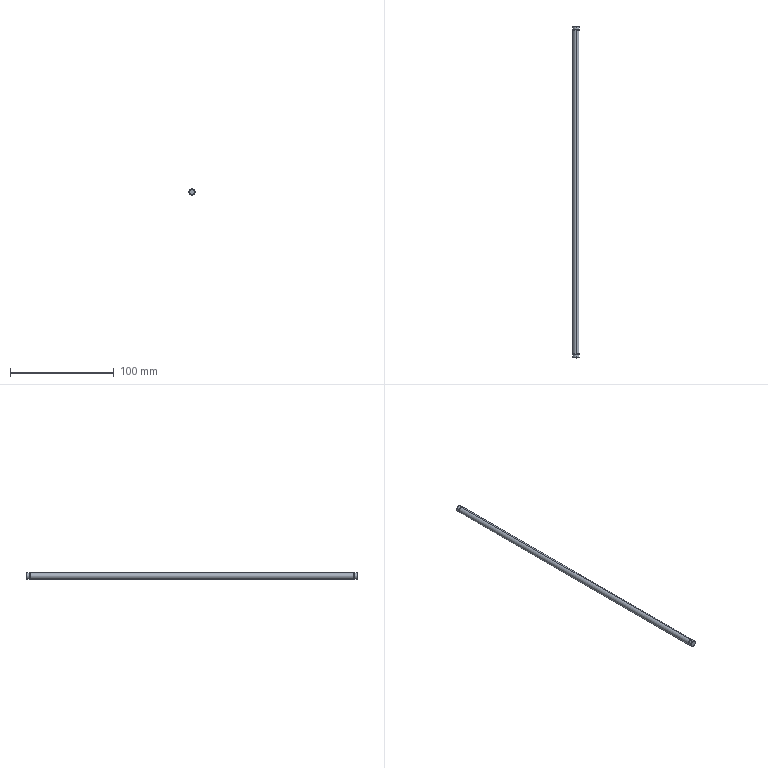Part | STEP file | 6mm pin shaft 001 | 1 solid | 20 faces | box 6 x 320 x 6 mm | volume 9038 mm3 | cylinder 10 | plane 6 | cone 4 | commonest cylinder face diameters 6 x6 5.6 x4
STEP:
#1=CARTESIAN_POINT('',(0.,0.,0.));
#2=DIRECTION('',(0.,0.,1.));
#3=DIRECTION('',(1.,0.,0.));
#4=AXIS2_PLACEMENT_3D('',#1,#2,#3);
#5=CARTESIAN_POINT('',(0.,-160.,-2.5));
#6=VERTEX_POINT('',#5);
#7=CARTESIAN_POINT('',(0.,-160.,2.5));
#8=VERTEX_POINT('',#7);
#9=CARTESIAN_POINT('',(0.,-160.,0.));
#10=DIRECTION('',(0.,-1.,0.));
#11=DIRECTION('',(0.,0.,1.));
#12=AXIS2_PLACEMENT_3D('',#9,#10,#11);
#13=CIRCLE('',#12,2.5);
#14=CARTESIAN_POINT('',(0.,-159.5,0.));
#15=DIRECTION('',(0.,1.,0.));
#16=DIRECTION('',(0.,0.,1.));
#17=AXIS2_PLACEMENT_3D('',#14,#15,#16);
#18=CONICAL_SURFACE('',#17,3.,0.7854);
#19=CARTESIAN_POINT('',(6.283,-0.5));
#20=DIRECTION('',(-1.,0.));
#21=VECTOR('',#20,1.);
#22=LINE('',#19,#21);
#23=(GEOMETRIC_REPRESENTATION_CONTEXT(2)PARAMETRIC_REPRESENTATION_CONTEXT()REPRESENTATION_CONTEXT('',''));
#24=DEFINITIONAL_REPRESENTATION('',(#22),#23);
#25=PCURVE('',#18,#24);
#26=CARTESIAN_POINT('',(0.,-160.,0.));
#27=DIRECTION('',(0.,1.,0.));
#28=DIRECTION('',(0.,0.,1.));
#29=AXIS2_PLACEMENT_3D('',#26,#27,#28);
#30=PLANE('',#29);
#31=CARTESIAN_POINT('',(2.5,0.));
#32=CARTESIAN_POINT('',(2.5,-4.33));
#33=CARTESIAN_POINT('',(-1.25,-2.165));
#34=CARTESIAN_POINT('',(-5.,0.));
#35=CARTESIAN_POINT('',(-1.25,2.165));
#36=CARTESIAN_POINT('',(2.5,4.33));
#37=CARTESIAN_POINT('',(2.5,0.));
#38=(BOUNDED_CURVE()B_SPLINE_CURVE(2,(#31,#32,#33,#34,#35,#36,#37),.UNSPECIFIED.,.T.,.F.)B_SPLINE_CURVE_WITH_KNOTS((1,2,2,2,2,1),(-2.094,0.,2.094,4.189,6.283,8.378),.UNSPECIFIED.)CURVE()GEOMETRIC_REPRESENTATION_ITEM()RATIONAL_B_SPLINE_CURVE((1.,0.5,1.,0.5,1.,0.5,1.))REPRESENTATION_ITEM(''));
#39=(GEOMETRIC_REPRESENTATION_CONTEXT(2)PARAMETRIC_REPRESENTATION_CONTEXT()REPRESENTATION_CONTEXT('',''));
#40=DEFINITIONAL_REPRESENTATION('',(#38),#39);
#41=PCURVE('',#30,#40);
#42=SURFACE_CURVE('',#13,(#25,#41),.PCURVE_S1.);
#43=EDGE_CURVE('',#6,#8,#42,.T.);
#44=ORIENTED_EDGE('',*,*,#43,.F.);
#45=CARTESIAN_POINT('',(0.,-159.5,-3.));
#46=VERTEX_POINT('',#45);
#47=CARTESIAN_POINT('',(0.,-159.5,-3.));
#48=DIRECTION('',(0.,0.7071,-0.7071));
#49=VECTOR('',#48,1.);
#50=LINE('',#47,#49);
#51=CARTESIAN_POINT('',(3.142,0.));
#52=DIRECTION('',(0.,1.));
#53=VECTOR('',#52,1.);
#54=LINE('',#51,#53);
#55=(GEOMETRIC_REPRESENTATION_CONTEXT(2)PARAMETRIC_REPRESENTATION_CONTEXT()REPRESENTATION_CONTEXT('',''));
#56=DEFINITIONAL_REPRESENTATION('',(#54),#55);
#57=PCURVE('',#18,#56);
#58=CARTESIAN_POINT('',(0.,-159.5,0.));
#59=DIRECTION('',(0.,1.,0.));
#60=DIRECTION('',(0.,0.,1.));
#61=AXIS2_PLACEMENT_3D('',#58,#59,#60);
#62=CONICAL_SURFACE('',#61,3.,0.7854);
#63=CARTESIAN_POINT('',(3.142,0.));
#64=DIRECTION('',(0.,1.));
#65=VECTOR('',#64,1.);
#66=LINE('',#63,#65);
#67=(GEOMETRIC_REPRESENTATION_CONTEXT(2)PARAMETRIC_REPRESENTATION_CONTEXT()REPRESENTATION_CONTEXT('',''));
#68=DEFINITIONAL_REPRESENTATION('',(#66),#67);
#69=PCURVE('',#62,#68);
#70=SURFACE_CURVE('',#50,(#57,#69),.PCURVE_S1.);
#71=EDGE_CURVE('',#6,#46,#70,.T.);
#72=ORIENTED_EDGE('',*,*,#71,.T.);
#73=CARTESIAN_POINT('',(0.,-159.5,3.));
#74=VERTEX_POINT('',#73);
#75=CARTESIAN_POINT('',(0.,-159.5,0.));
#76=DIRECTION('',(0.,1.,0.));
#77=DIRECTION('',(0.,0.,1.));
#78=AXIS2_PLACEMENT_3D('',#75,#76,#77);
#79=CIRCLE('',#78,3.);
#80=CARTESIAN_POINT('',(0.,0.));
#81=DIRECTION('',(1.,0.));
#82=VECTOR('',#81,1.);
#83=LINE('',#80,#82);
#84=(GEOMETRIC_REPRESENTATION_CONTEXT(2)PARAMETRIC_REPRESENTATION_CONTEXT()REPRESENTATION_CONTEXT('',''));
#85=DEFINITIONAL_REPRESENTATION('',(#83),#84);
#86=PCURVE('',#18,#85);
#87=CARTESIAN_POINT('',(0.,160.,0.));
#88=DIRECTION('',(0.,-1.,0.));
#89=DIRECTION('',(0.,0.,-1.));
#90=AXIS2_PLACEMENT_3D('',#87,#88,#89);
#91=CYLINDRICAL_SURFACE('',#90,3.);
#92=CARTESIAN_POINT('',(3.142,319.5));
#93=DIRECTION('',(-1.,0.));
#94=VECTOR('',#93,1.);
#95=LINE('',#92,#94);
#96=(GEOMETRIC_REPRESENTATION_CONTEXT(2)PARAMETRIC_REPRESENTATION_CONTEXT()REPRESENTATION_CONTEXT('',''));
#97=DEFINITIONAL_REPRESENTATION('',(#95),#96);
#98=PCURVE('',#91,#97);
#99=SURFACE_CURVE('',#79,(#86,#98),.PCURVE_S1.);
#100=EDGE_CURVE('',#74,#46,#99,.T.);
#101=ORIENTED_EDGE('',*,*,#100,.F.);
#102=CARTESIAN_POINT('',(0.,-159.5,3.));
#103=DIRECTION('',(0.,0.7071,0.7071));
#104=VECTOR('',#103,1.);
#105=LINE('',#102,#104);
#106=CARTESIAN_POINT('',(0.,0.));
#107=DIRECTION('',(0.,1.));
#108=VECTOR('',#107,1.);
#109=LINE('',#106,#108);
#110=(GEOMETRIC_REPRESENTATION_CONTEXT(2)PARAMETRIC_REPRESENTATION_CONTEXT()REPRESENTATION_CONTEXT('',''));
#111=DEFINITIONAL_REPRESENTATION('',(#109),#110);
#112=PCURVE('',#18,#111);
#113=CARTESIAN_POINT('',(6.283,0.));
#114=DIRECTION('',(0.,1.));
#115=VECTOR('',#114,1.);
#116=LINE('',#113,#115);
#117=(GEOMETRIC_REPRESENTATION_CONTEXT(2)PARAMETRIC_REPRESENTATION_CONTEXT()REPRESENTATION_CONTEXT('',''));
#118=DEFINITIONAL_REPRESENTATION('',(#116),#117);
#119=PCURVE('',#62,#118);
#120=SURFACE_CURVE('',#105,(#112,#119),.PCURVE_S1.);
#121=EDGE_CURVE('',#8,#74,#120,.T.);
#122=ORIENTED_EDGE('',*,*,#121,.F.);
#123=EDGE_LOOP('',(#44,#72,#101,#122));
#124=FACE_BOUND('',#123,.T.);
#125=ADVANCED_FACE('',(#124),#18,.T.);
#126=CARTESIAN_POINT('',(0.,160.,2.5));
#127=VERTEX_POINT('',#126);
#128=CARTESIAN_POINT('',(0.,160.,-2.5));
#129=VERTEX_POINT('',#128);
#130=CARTESIAN_POINT('',(0.,160.,0.));
#131=DIRECTION('',(0.,1.,0.));
#132=DIRECTION('',(0.,0.,1.));
#133=AXIS2_PLACEMENT_3D('',#130,#131,#132);
#134=CIRCLE('',#133,2.5);
#135=CARTESIAN_POINT('',(0.,160.,0.));
#136=DIRECTION('',(0.,-1.,0.));
#137=DIRECTION('',(0.,0.,-1.));
#138=AXIS2_PLACEMENT_3D('',#135,#136,#137);
#139=CONICAL_SURFACE('',#138,2.5,0.7854);
#140=CARTESIAN_POINT('',(3.142,0.));
#141=DIRECTION('',(-1.,0.));
#142=VECTOR('',#141,1.);
#143=LINE('',#140,#142);
#144=(GEOMETRIC_REPRESENTATION_CONTEXT(2)PARAMETRIC_REPRESENTATION_CONTEXT()REPRESENTATION_CONTEXT('',''));
#145=DEFINITIONAL_REPRESENTATION('',(#143),#144);
#146=PCURVE('',#139,#145);
#147=CARTESIAN_POINT('',(0.,160.,0.));
#148=DIRECTION('',(0.,1.,0.));
#149=DIRECTION('',(0.,0.,1.));
#150=AXIS2_PLACEMENT_3D('',#147,#148,#149);
#151=PLANE('',#150);
#152=CARTESIAN_POINT('',(0.,0.));
#153=DIRECTION('',(1.,0.));
#154=AXIS2_PLACEMENT_2D('',#152,#153);
#155=CIRCLE('',#154,2.5);
#156=(GEOMETRIC_REPRESENTATION_CONTEXT(2)PARAMETRIC_REPRESENTATION_CONTEXT()REPRESENTATION_CONTEXT('',''));
#157=DEFINITIONAL_REPRESENTATION('',(#155),#156);
#158=PCURVE('',#151,#157);
#159=SURFACE_CURVE('',#134,(#146,#158),.PCURVE_S1.);
#160=EDGE_CURVE('',#127,#129,#159,.T.);
#161=ORIENTED_EDGE('',*,*,#160,.F.);
#162=CARTESIAN_POINT('',(0.,159.5,3.));
#163=VERTEX_POINT('',#162);
#164=CARTESIAN_POINT('',(0.,160.,2.5));
#165=DIRECTION('',(0.,-0.7071,0.7071));
#166=VECTOR('',#165,1.);
#167=LINE('',#164,#166);
#168=CARTESIAN_POINT('',(3.142,0.));
#169=DIRECTION('',(0.,1.));
#170=VECTOR('',#169,1.);
#171=LINE('',#168,#170);
#172=(GEOMETRIC_REPRESENTATION_CONTEXT(2)PARAMETRIC_REPRESENTATION_CONTEXT()REPRESENTATION_CONTEXT('',''));
#173=DEFINITIONAL_REPRESENTATION('',(#171),#172);
#174=PCURVE('',#139,#173);
#175=CARTESIAN_POINT('',(0.,160.,0.));
#176=DIRECTION('',(0.,-1.,0.));
#177=DIRECTION('',(0.,0.,-1.));
#178=AXIS2_PLACEMENT_3D('',#175,#176,#177);
#179=CONICAL_SURFACE('',#178,2.5,0.7854);
#180=CARTESIAN_POINT('',(3.142,0.));
#181=DIRECTION('',(0.,1.));
#182=VECTOR('',#181,1.);
#183=LINE('',#180,#182);
#184=(GEOMETRIC_REPRESENTATION_CONTEXT(2)PARAMETRIC_REPRESENTATION_CONTEXT()REPRESENTATION_CONTEXT('',''));
#185=DEFINITIONAL_REPRESENTATION('',(#183),#184);
#186=PCURVE('',#179,#185);
#187=SURFACE_CURVE('',#167,(#174,#186),.PCURVE_S1.);
#188=EDGE_CURVE('',#127,#163,#187,.T.);
#189=ORIENTED_EDGE('',*,*,#188,.T.);
#190=CARTESIAN_POINT('',(0.,159.5,-3.));
#191=VERTEX_POINT('',#190);
#192=CARTESIAN_POINT('',(0.,159.5,0.));
#193=DIRECTION('',(0.,-1.,0.));
#194=DIRECTION('',(0.,0.,1.));
#195=AXIS2_PLACEMENT_3D('',#192,#193,#194);
#196=CIRCLE('',#195,3.);
#197=CARTESIAN_POINT('',(-3.142,0.5));
#198=DIRECTION('',(1.,0.));
#199=VECTOR('',#198,1.);
#200=LINE('',#197,#199);
#201=(GEOMETRIC_REPRESENTATION_CONTEXT(2)PARAMETRIC_REPRESENTATION_CONTEXT()REPRESENTATION_CONTEXT('',''));
#202=DEFINITIONAL_REPRESENTATION('',(#200),#201);
#203=PCURVE('',#139,#202);
#204=CARTESIAN_POINT('',(0.,160.,0.));
#205=DIRECTION('',(0.,-1.,0.));
#206=DIRECTION('',(0.,0.,-1.));
#207=AXIS2_PLACEMENT_3D('',#204,#205,#206);
#208=CYLINDRICAL_SURFACE('',#207,3.);
#209=CARTESIAN_POINT('',(-3.142,0.5));
#210=DIRECTION('',(1.,0.));
#211=VECTOR('',#210,1.);
#212=LINE('',#209,#211);
#213=(GEOMETRIC_REPRESENTATION_CONTEXT(2)PARAMETRIC_REPRESENTATION_CONTEXT()REPRESENTATION_CONTEXT('',''));
#214=DEFINITIONAL_REPRESENTATION('',(#212),#213);
#215=PCURVE('',#208,#214);
#216=SURFACE_CURVE('',#196,(#203,#215),.PCURVE_S1.);
#217=EDGE_CURVE('',#191,#163,#216,.T.);
#218=ORIENTED_EDGE('',*,*,#217,.F.);
#219=CARTESIAN_POINT('',(0.,160.,-2.5));
#220=DIRECTION('',(0.,-0.7071,-0.7071));
#221=VECTOR('',#220,1.);
#222=LINE('',#219,#221);
#223=CARTESIAN_POINT('',(0.,0.));
#224=DIRECTION('',(0.,1.));
#225=VECTOR('',#224,1.);
#226=LINE('',#223,#225);
#227=(GEOMETRIC_REPRESENTATION_CONTEXT(2)PARAMETRIC_REPRESENTATION_CONTEXT()REPRESENTATION_CONTEXT('',''));
#228=DEFINITIONAL_REPRESENTATION('',(#226),#227);
#229=PCURVE('',#139,#228);
#230=CARTESIAN_POINT('',(6.283,0.));
#231=DIRECTION('',(0.,1.));
#232=VECTOR('',#231,1.);
#233=LINE('',#230,#232);
#234=(GEOMETRIC_REPRESENTATION_CONTEXT(2)PARAMETRIC_REPRESENTATION_CONTEXT()REPRESENTATION_CONTEXT('',''));
#235=DEFINITIONAL_REPRESENTATION('',(#233),#234);
#236=PCURVE('',#179,#235);
#237=SURFACE_CURVE('',#222,(#229,#236),.PCURVE_S1.);
#238=EDGE_CURVE('',#129,#191,#237,.T.);
#239=ORIENTED_EDGE('',*,*,#238,.F.);
#240=EDGE_LOOP('',(#161,#189,#218,#239));
#241=FACE_BOUND('',#240,.T.);
#242=ADVANCED_FACE('',(#241),#139,.T.);
#243=CARTESIAN_POINT('',(0.,-156.7,3.));
#244=VERTEX_POINT('',#243);
#245=CARTESIAN_POINT('',(0.,-156.7,-3.));
#246=VERTEX_POINT('',#245);
#247=CARTESIAN_POINT('',(0.,-156.7,0.));
#248=DIRECTION('',(0.,1.,0.));
#249=DIRECTION('',(0.,0.,1.));
#250=AXIS2_PLACEMENT_3D('',#247,#248,#249);
#251=CIRCLE('',#250,3.);
#252=CARTESIAN_POINT('',(3.142,316.7));
#253=DIRECTION('',(-1.,0.));
#254=VECTOR('',#253,1.);
#255=LINE('',#252,#254);
#256=(GEOMETRIC_REPRESENTATION_CONTEXT(2)PARAMETRIC_REPRESENTATION_CONTEXT()REPRESENTATION_CONTEXT('',''));
#257=DEFINITIONAL_REPRESENTATION('',(#255),#256);
#258=PCURVE('',#91,#257);
#259=CARTESIAN_POINT('',(-5.32,-156.7,0.));
#260=DIRECTION('',(0.,1.,0.));
#261=DIRECTION('',(0.,0.,1.));
#262=AXIS2_PLACEMENT_3D('',#259,#260,#261);
#263=PLANE('',#262);
#264=CARTESIAN_POINT('',(0.,5.32));
#265=DIRECTION('',(1.,0.));
#266=AXIS2_PLACEMENT_2D('',#264,#265);
#267=CIRCLE('',#266,3.);
#268=(GEOMETRIC_REPRESENTATION_CONTEXT(2)PARAMETRIC_REPRESENTATION_CONTEXT()REPRESENTATION_CONTEXT('',''));
#269=DEFINITIONAL_REPRESENTATION('',(#267),#268);
#270=PCURVE('',#263,#269);
#271=SURFACE_CURVE('',#251,(#258,#270),.PCURVE_S1.);
#272=EDGE_CURVE('',#244,#246,#271,.T.);
#273=ORIENTED_EDGE('',*,*,#272,.F.);
#274=CARTESIAN_POINT('',(0.,160.,3.));
#275=DIRECTION('',(0.,-1.,0.));
#276=VECTOR('',#275,1.);
#277=LINE('',#274,#276);
#278=CARTESIAN_POINT('',(3.142,0.));
#279=DIRECTION('',(0.,1.));
#280=VECTOR('',#279,1.);
#281=LINE('',#278,#280);
#282=(GEOMETRIC_REPRESENTATION_CONTEXT(2)PARAMETRIC_REPRESENTATION_CONTEXT()REPRESENTATION_CONTEXT('',''));
#283=DEFINITIONAL_REPRESENTATION('',(#281),#282);
#284=PCURVE('',#91,#283);
#285=CARTESIAN_POINT('',(0.,160.,0.));
#286=DIRECTION('',(0.,-1.,0.));
#287=DIRECTION('',(0.,0.,-1.));
#288=AXIS2_PLACEMENT_3D('',#285,#286,#287);
#289=CYLINDRICAL_SURFACE('',#288,3.);
#290=CARTESIAN_POINT('',(3.142,0.));
#291=DIRECTION('',(0.,1.));
#292=VECTOR('',#291,1.);
#293=LINE('',#290,#292);
#294=(GEOMETRIC_REPRESENTATION_CONTEXT(2)PARAMETRIC_REPRESENTATION_CONTEXT()REPRESENTATION_CONTEXT('',''));
#295=DEFINITIONAL_REPRESENTATION('',(#293),#294);
#296=PCURVE('',#289,#295);
#297=SURFACE_CURVE('',#277,(#284,#296),.PCURVE_S1.);
#298=EDGE_CURVE('',#244,#74,#297,.T.);
#299=ORIENTED_EDGE('',*,*,#298,.T.);
#300=ORIENTED_EDGE('',*,*,#100,.T.);
#301=CARTESIAN_POINT('',(0.,160.,-3.));
#302=DIRECTION('',(0.,-1.,0.));
#303=VECTOR('',#302,1.);
#304=LINE('',#301,#303);
#305=CARTESIAN_POINT('',(0.,0.));
#306=DIRECTION('',(0.,1.));
#307=VECTOR('',#306,1.);
#308=LINE('',#305,#307);
#309=(GEOMETRIC_REPRESENTATION_CONTEXT(2)PARAMETRIC_REPRESENTATION_CONTEXT()REPRESENTATION_CONTEXT('',''));
#310=DEFINITIONAL_REPRESENTATION('',(#308),#309);
#311=PCURVE('',#91,#310);
#312=CARTESIAN_POINT('',(6.283,0.));
#313=DIRECTION('',(0.,1.));
#314=VECTOR('',#313,1.);
#315=LINE('',#312,#314);
#316=(GEOMETRIC_REPRESENTATION_CONTEXT(2)PARAMETRIC_REPRESENTATION_CONTEXT()REPRESENTATION_CONTEXT('',''));
#317=DEFINITIONAL_REPRESENTATION('',(#315),#316);
#318=PCURVE('',#289,#317);
#319=SURFACE_CURVE('',#304,(#311,#318),.PCURVE_S1.);
#320=EDGE_CURVE('',#246,#46,#319,.T.);
#321=ORIENTED_EDGE('',*,*,#320,.F.);
#322=EDGE_LOOP('',(#273,#299,#300,#321));
#323=FACE_BOUND('',#322,.T.);
#324=ADVANCED_FACE('',(#323),#91,.T.);
#325=CARTESIAN_POINT('',(0.,-156.,-2.8));
#326=VERTEX_POINT('',#325);
#327=CARTESIAN_POINT('',(0.,-156.,2.8));
#328=VERTEX_POINT('',#327);
#329=CARTESIAN_POINT('',(0.,-156.,0.));
#330=DIRECTION('',(0.,-1.,0.));
#331=DIRECTION('',(0.,0.,-1.));
#332=AXIS2_PLACEMENT_3D('',#329,#330,#331);
#333=CIRCLE('',#332,2.8);
#334=CARTESIAN_POINT('',(0.,0.,0.));
#335=DIRECTION('',(0.,-1.,0.));
#336=DIRECTION('',(0.,0.,-1.));
#337=AXIS2_PLACEMENT_3D('',#334,#335,#336);
#338=CYLINDRICAL_SURFACE('',#337,2.8);
#339=CARTESIAN_POINT('',(0.,156.));
#340=DIRECTION('',(1.,0.));
#341=VECTOR('',#340,1.);
#342=LINE('',#339,#341);
#343=(GEOMETRIC_REPRESENTATION_CONTEXT(2)PARAMETRIC_REPRESENTATION_CONTEXT()REPRESENTATION_CONTEXT('',''));
#344=DEFINITIONAL_REPRESENTATION('',(#342),#343);
#345=PCURVE('',#338,#344);
#346=CARTESIAN_POINT('',(-5.32,-156.,0.));
#347=DIRECTION('',(0.,-1.,0.));
#348=DIRECTION('',(0.,0.,-1.));
#349=AXIS2_PLACEMENT_3D('',#346,#347,#348);
#350=PLANE('',#349);
#351=CARTESIAN_POINT('',(0.,5.32));
#352=DIRECTION('',(1.,0.));
#353=AXIS2_PLACEMENT_2D('',#351,#352);
#354=CIRCLE('',#353,2.8);
#355=(GEOMETRIC_REPRESENTATION_CONTEXT(2)PARAMETRIC_REPRESENTATION_CONTEXT()REPRESENTATION_CONTEXT('',''));
#356=DEFINITIONAL_REPRESENTATION('',(#354),#355);
#357=PCURVE('',#350,#356);
#358=SURFACE_CURVE('',#333,(#345,#357),.PCURVE_S1.);
#359=EDGE_CURVE('',#326,#328,#358,.T.);
#360=ORIENTED_EDGE('',*,*,#359,.T.);
#361=CARTESIAN_POINT('',(0.,-156.7,2.8));
#362=VERTEX_POINT('',#361);
#363=CARTESIAN_POINT('',(0.,0.,2.8));
#364=DIRECTION('',(0.,-1.,0.));
#365=VECTOR('',#364,1.);
#366=LINE('',#363,#365);
#367=CARTESIAN_POINT('',(3.142,0.));
#368=DIRECTION('',(0.,1.));
#369=VECTOR('',#368,1.);
#370=LINE('',#367,#369);
#371=(GEOMETRIC_REPRESENTATION_CONTEXT(2)PARAMETRIC_REPRESENTATION_CONTEXT()REPRESENTATION_CONTEXT('',''));
#372=DEFINITIONAL_REPRESENTATION('',(#370),#371);
#373=PCURVE('',#338,#372);
#374=CARTESIAN_POINT('',(0.,0.,0.));
#375=DIRECTION('',(0.,-1.,0.));
#376=DIRECTION('',(0.,0.,-1.));
#377=AXIS2_PLACEMENT_3D('',#374,#375,#376);
#378=CYLINDRICAL_SURFACE('',#377,2.8);
#379=CARTESIAN_POINT('',(3.142,0.));
#380=DIRECTION('',(0.,1.));
#381=VECTOR('',#380,1.);
#382=LINE('',#379,#381);
#383=(GEOMETRIC_REPRESENTATION_CONTEXT(2)PARAMETRIC_REPRESENTATION_CONTEXT()REPRESENTATION_CONTEXT('',''));
#384=DEFINITIONAL_REPRESENTATION('',(#382),#383);
#385=PCURVE('',#378,#384);
#386=SURFACE_CURVE('',#366,(#373,#385),.PCURVE_S1.);
#387=EDGE_CURVE('',#328,#362,#386,.T.);
#388=ORIENTED_EDGE('',*,*,#387,.T.);
#389=CARTESIAN_POINT('',(0.,-156.7,-2.8));
#390=VERTEX_POINT('',#389);
#391=CARTESIAN_POINT('',(0.,-156.7,0.));
#392=DIRECTION('',(0.,-1.,0.));
#393=DIRECTION('',(0.,0.,-1.));
#394=AXIS2_PLACEMENT_3D('',#391,#392,#393);
#395=CIRCLE('',#394,2.8);
#396=CARTESIAN_POINT('',(0.,156.7));
#397=DIRECTION('',(1.,0.));
#398=VECTOR('',#397,1.);
#399=LINE('',#396,#398);
#400=(GEOMETRIC_REPRESENTATION_CONTEXT(2)PARAMETRIC_REPRESENTATION_CONTEXT()REPRESENTATION_CONTEXT('',''));
#401=DEFINITIONAL_REPRESENTATION('',(#399),#400);
#402=PCURVE('',#338,#401);
#403=CARTESIAN_POINT('',(-2.8,5.32));
#404=CARTESIAN_POINT('',(-2.8,10.17));
#405=CARTESIAN_POINT('',(1.4,7.745));
#406=CARTESIAN_POINT('',(5.6,5.32));
#407=CARTESIAN_POINT('',(1.4,2.895));
#408=CARTESIAN_POINT('',(-2.8,0.4702));
#409=CARTESIAN_POINT('',(-2.8,5.32));
#410=(BOUNDED_CURVE()B_SPLINE_CURVE(2,(#403,#404,#405,#406,#407,#408,#409),.UNSPECIFIED.,.T.,.F.)B_SPLINE_CURVE_WITH_KNOTS((1,2,2,2,2,1),(-2.094,0.,2.094,4.189,6.283,8.378),.UNSPECIFIED.)CURVE()GEOMETRIC_REPRESENTATION_ITEM()RATIONAL_B_SPLINE_CURVE((1.,0.5,1.,0.5,1.,0.5,1.))REPRESENTATION_ITEM(''));
#411=(GEOMETRIC_REPRESENTATION_CONTEXT(2)PARAMETRIC_REPRESENTATION_CONTEXT()REPRESENTATION_CONTEXT('',''));
#412=DEFINITIONAL_REPRESENTATION('',(#410),#411);
#413=PCURVE('',#263,#412);
#414=SURFACE_CURVE('',#395,(#402,#413),.PCURVE_S1.);
#415=EDGE_CURVE('',#390,#362,#414,.T.);
#416=ORIENTED_EDGE('',*,*,#415,.F.);
#417=CARTESIAN_POINT('',(0.,0.,-2.8));
#418=DIRECTION('',(0.,-1.,0.));
#419=VECTOR('',#418,1.);
#420=LINE('',#417,#419);
#421=CARTESIAN_POINT('',(0.,0.));
#422=DIRECTION('',(0.,1.));
#423=VECTOR('',#422,1.);
#424=LINE('',#421,#423);
#425=(GEOMETRIC_REPRESENTATION_CONTEXT(2)PARAMETRIC_REPRESENTATION_CONTEXT()REPRESENTATION_CONTEXT('',''));
#426=DEFINITIONAL_REPRESENTATION('',(#424),#425);
#427=PCURVE('',#338,#426);
#428=CARTESIAN_POINT('',(6.283,0.));
#429=DIRECTION('',(0.,1.));
#430=VECTOR('',#429,1.);
#431=LINE('',#428,#430);
#432=(GEOMETRIC_REPRESENTATION_CONTEXT(2)PARAMETRIC_REPRESENTATION_CONTEXT()REPRESENTATION_CONTEXT('',''));
#433=DEFINITIONAL_REPRESENTATION('',(#431),#432);
#434=PCURVE('',#378,#433);
#435=SURFACE_CURVE('',#420,(#427,#434),.PCURVE_S1.);
#436=EDGE_CURVE('',#326,#390,#435,.T.);
#437=ORIENTED_EDGE('',*,*,#436,.F.);
#438=EDGE_LOOP('',(#360,#388,#416,#437));
#439=FACE_BOUND('',#438,.T.);
#440=ADVANCED_FACE('',(#439),#338,.T.);
#441=CARTESIAN_POINT('',(0.,156.,3.));
#442=VERTEX_POINT('',#441);
#443=CARTESIAN_POINT('',(0.,156.,-3.));
#444=VERTEX_POINT('',#443);
#445=CARTESIAN_POINT('',(0.,156.,0.));
#446=DIRECTION('',(0.,1.,0.));
#447=DIRECTION('',(0.,0.,1.));
#448=AXIS2_PLACEMENT_3D('',#445,#446,#447);
#449=CIRCLE('',#448,3.);
#450=CARTESIAN_POINT('',(0.,160.,0.));
#451=DIRECTION('',(0.,-1.,0.));
#452=DIRECTION('',(0.,0.,-1.));
#453=AXIS2_PLACEMENT_3D('',#450,#451,#452);
#454=CYLINDRICAL_SURFACE('',#453,3.);
#455=CARTESIAN_POINT('',(3.142,4.));
#456=DIRECTION('',(-1.,0.));
#457=VECTOR('',#456,1.);
#458=LINE('',#455,#457);
#459=(GEOMETRIC_REPRESENTATION_CONTEXT(2)PARAMETRIC_REPRESENTATION_CONTEXT()REPRESENTATION_CONTEXT('',''));
#460=DEFINITIONAL_REPRESENTATION('',(#458),#459);
#461=PCURVE('',#454,#460);
#462=CARTESIAN_POINT('',(-5.32,156.,0.));
#463=DIRECTION('',(0.,1.,0.));
#464=DIRECTION('',(0.,0.,1.));
#465=AXIS2_PLACEMENT_3D('',#462,#463,#464);
#466=PLANE('',#465);
#467=CARTESIAN_POINT('',(0.,5.32));
#468=DIRECTION('',(1.,0.));
#469=AXIS2_PLACEMENT_2D('',#467,#468);
#470=CIRCLE('',#469,3.);
#471=(GEOMETRIC_REPRESENTATION_CONTEXT(2)PARAMETRIC_REPRESENTATION_CONTEXT()REPRESENTATION_CONTEXT('',''));
#472=DEFINITIONAL_REPRESENTATION('',(#470),#471);
#473=PCURVE('',#466,#472);
#474=SURFACE_CURVE('',#449,(#461,#473),.PCURVE_S1.);
#475=EDGE_CURVE('',#442,#444,#474,.T.);
#476=ORIENTED_EDGE('',*,*,#475,.F.);
#477=CARTESIAN_POINT('',(0.,-156.,3.));
#478=VERTEX_POINT('',#477);
#479=CARTESIAN_POINT('',(0.,160.,3.));
#480=DIRECTION('',(0.,-1.,0.));
#481=VECTOR('',#480,1.);
#482=LINE('',#479,#481);
#483=CARTESIAN_POINT('',(3.142,0.));
#484=DIRECTION('',(0.,1.));
#485=VECTOR('',#484,1.);
#486=LINE('',#483,#485);
#487=(GEOMETRIC_REPRESENTATION_CONTEXT(2)PARAMETRIC_REPRESENTATION_CONTEXT()REPRESENTATION_CONTEXT('',''));
#488=DEFINITIONAL_REPRESENTATION('',(#486),#487);
#489=PCURVE('',#454,#488);
#490=CARTESIAN_POINT('',(0.,160.,0.));
#491=DIRECTION('',(0.,-1.,0.));
#492=DIRECTION('',(0.,0.,-1.));
#493=AXIS2_PLACEMENT_3D('',#490,#491,#492);
#494=CYLINDRICAL_SURFACE('',#493,3.);
#495=CARTESIAN_POINT('',(3.142,0.));
#496=DIRECTION('',(0.,1.));
#497=VECTOR('',#496,1.);
#498=LINE('',#495,#497);
#499=(GEOMETRIC_REPRESENTATION_CONTEXT(2)PARAMETRIC_REPRESENTATION_CONTEXT()REPRESENTATION_CONTEXT('',''));
#500=DEFINITIONAL_REPRESENTATION('',(#498),#499);
#501=PCURVE('',#494,#500);
#502=SURFACE_CURVE('',#482,(#489,#501),.PCURVE_S1.);
#503=EDGE_CURVE('',#442,#478,#502,.T.);
#504=ORIENTED_EDGE('',*,*,#503,.T.);
#505=CARTESIAN_POINT('',(0.,-156.,-3.));
#506=VERTEX_POINT('',#505);
#507=CARTESIAN_POINT('',(0.,-156.,0.));
#508=DIRECTION('',(0.,-1.,0.));
#509=DIRECTION('',(0.,0.,-1.));
#510=AXIS2_PLACEMENT_3D('',#507,#508,#509);
#511=CIRCLE('',#510,3.);
#512=CARTESIAN_POINT('',(0.,316.));
#513=DIRECTION('',(1.,0.));
#514=VECTOR('',#513,1.);
#515=LINE('',#512,#514);
#516=(GEOMETRIC_REPRESENTATION_CONTEXT(2)PARAMETRIC_REPRESENTATION_CONTEXT()REPRESENTATION_CONTEXT('',''));
#517=DEFINITIONAL_REPRESENTATION('',(#515),#516);
#518=PCURVE('',#454,#517);
#519=CARTESIAN_POINT('',(0.,5.32));
#520=DIRECTION('',(1.,0.));
#521=AXIS2_PLACEMENT_2D('',#519,#520);
#522=CIRCLE('',#521,3.);
#523=(GEOMETRIC_REPRESENTATION_CONTEXT(2)PARAMETRIC_REPRESENTATION_CONTEXT()REPRESENTATION_CONTEXT('',''));
#524=DEFINITIONAL_REPRESENTATION('',(#522),#523);
#525=PCURVE('',#350,#524);
#526=SURFACE_CURVE('',#511,(#518,#525),.PCURVE_S1.);
#527=EDGE_CURVE('',#506,#478,#526,.T.);
#528=ORIENTED_EDGE('',*,*,#527,.F.);
#529=CARTESIAN_POINT('',(0.,160.,-3.));
#530=DIRECTION('',(0.,-1.,0.));
#531=VECTOR('',#530,1.);
#532=LINE('',#529,#531);
#533=CARTESIAN_POINT('',(0.,0.));
#534=DIRECTION('',(0.,1.));
#535=VECTOR('',#534,1.);
#536=LINE('',#533,#535);
#537=(GEOMETRIC_REPRESENTATION_CONTEXT(2)PARAMETRIC_REPRESENTATION_CONTEXT()REPRESENTATION_CONTEXT('',''));
#538=DEFINITIONAL_REPRESENTATION('',(#536),#537);
#539=PCURVE('',#454,#538);
#540=CARTESIAN_POINT('',(6.283,0.));
#541=DIRECTION('',(0.,1.));
#542=VECTOR('',#541,1.);
#543=LINE('',#540,#542);
#544=(GEOMETRIC_REPRESENTATION_CONTEXT(2)PARAMETRIC_REPRESENTATION_CONTEXT()REPRESENTATION_CONTEXT('',''));
#545=DEFINITIONAL_REPRESENTATION('',(#543),#544);
#546=PCURVE('',#494,#545);
#547=SURFACE_CURVE('',#532,(#539,#546),.PCURVE_S1.);
#548=EDGE_CURVE('',#444,#506,#547,.T.);
#549=ORIENTED_EDGE('',*,*,#548,.F.);
#550=EDGE_LOOP('',(#476,#504,#528,#549));
#551=FACE_BOUND('',#550,.T.);
#552=ADVANCED_FACE('',(#551),#454,.T.);
#553=CARTESIAN_POINT('',(0.,156.7,-2.8));
#554=VERTEX_POINT('',#553);
#555=CARTESIAN_POINT('',(0.,156.7,2.8));
#556=VERTEX_POINT('',#555);
#557=CARTESIAN_POINT('',(0.,156.7,0.));
#558=DIRECTION('',(0.,-1.,0.));
#559=DIRECTION('',(0.,0.,-1.));
#560=AXIS2_PLACEMENT_3D('',#557,#558,#559);
#561=CIRCLE('',#560,2.8);
#562=CARTESIAN_POINT('',(0.,0.,0.));
#563=DIRECTION('',(0.,-1.,0.));
#564=DIRECTION('',(0.,0.,-1.));
#565=AXIS2_PLACEMENT_3D('',#562,#563,#564);
#566=CYLINDRICAL_SURFACE('',#565,2.8);
#567=CARTESIAN_POINT('',(0.,-156.7));
#568=DIRECTION('',(1.,0.));
#569=VECTOR('',#568,1.);
#570=LINE('',#567,#569);
#571=(GEOMETRIC_REPRESENTATION_CONTEXT(2)PARAMETRIC_REPRESENTATION_CONTEXT()REPRESENTATION_CONTEXT('',''));
#572=DEFINITIONAL_REPRESENTATION('',(#570),#571);
#573=PCURVE('',#566,#572);
#574=CARTESIAN_POINT('',(-5.32,156.7,0.));
#575=DIRECTION('',(0.,-1.,0.));
#576=DIRECTION('',(0.,0.,-1.));
#577=AXIS2_PLACEMENT_3D('',#574,#575,#576);
#578=PLANE('',#577);
#579=CARTESIAN_POINT('',(0.,5.32));
#580=DIRECTION('',(1.,0.));
#581=AXIS2_PLACEMENT_2D('',#579,#580);
#582=CIRCLE('',#581,2.8);
#583=(GEOMETRIC_REPRESENTATION_CONTEXT(2)PARAMETRIC_REPRESENTATION_CONTEXT()REPRESENTATION_CONTEXT('',''));
#584=DEFINITIONAL_REPRESENTATION('',(#582),#583);
#585=PCURVE('',#578,#584);
#586=SURFACE_CURVE('',#561,(#573,#585),.PCURVE_S1.);
#587=EDGE_CURVE('',#554,#556,#586,.T.);
#588=ORIENTED_EDGE('',*,*,#587,.T.);
#589=CARTESIAN_POINT('',(0.,156.,2.8));
#590=VERTEX_POINT('',#589);
#591=CARTESIAN_POINT('',(0.,0.,2.8));
#592=DIRECTION('',(0.,-1.,0.));
#593=VECTOR('',#592,1.);
#594=LINE('',#591,#593);
#595=CARTESIAN_POINT('',(3.142,0.));
#596=DIRECTION('',(0.,1.));
#597=VECTOR('',#596,1.);
#598=LINE('',#595,#597);
#599=(GEOMETRIC_REPRESENTATION_CONTEXT(2)PARAMETRIC_REPRESENTATION_CONTEXT()REPRESENTATION_CONTEXT('',''));
#600=DEFINITIONAL_REPRESENTATION('',(#598),#599);
#601=PCURVE('',#566,#600);
#602=CARTESIAN_POINT('',(0.,0.,0.));
#603=DIRECTION('',(0.,-1.,0.));
#604=DIRECTION('',(0.,0.,-1.));
#605=AXIS2_PLACEMENT_3D('',#602,#603,#604);
#606=CYLINDRICAL_SURFACE('',#605,2.8);
#607=CARTESIAN_POINT('',(3.142,0.));
#608=DIRECTION('',(0.,1.));
#609=VECTOR('',#608,1.);
#610=LINE('',#607,#609);
#611=(GEOMETRIC_REPRESENTATION_CONTEXT(2)PARAMETRIC_REPRESENTATION_CONTEXT()REPRESENTATION_CONTEXT('',''));
#612=DEFINITIONAL_REPRESENTATION('',(#610),#611);
#613=PCURVE('',#606,#612);
#614=SURFACE_CURVE('',#594,(#601,#613),.PCURVE_S1.);
#615=EDGE_CURVE('',#556,#590,#614,.T.);
#616=ORIENTED_EDGE('',*,*,#615,.T.);
#617=CARTESIAN_POINT('',(0.,156.,-2.8));
#618=VERTEX_POINT('',#617);
#619=CARTESIAN_POINT('',(0.,156.,0.));
#620=DIRECTION('',(0.,-1.,0.));
#621=DIRECTION('',(0.,0.,-1.));
#622=AXIS2_PLACEMENT_3D('',#619,#620,#621);
#623=CIRCLE('',#622,2.8);
#624=CARTESIAN_POINT('',(0.,-156.));
#625=DIRECTION('',(1.,0.));
#626=VECTOR('',#625,1.);
#627=LINE('',#624,#626);
#628=(GEOMETRIC_REPRESENTATION_CONTEXT(2)PARAMETRIC_REPRESENTATION_CONTEXT()REPRESENTATION_CONTEXT('',''));
#629=DEFINITIONAL_REPRESENTATION('',(#627),#628);
#630=PCURVE('',#566,#629);
#631=CARTESIAN_POINT('',(-2.8,5.32));
#632=CARTESIAN_POINT('',(-2.8,10.17));
#633=CARTESIAN_POINT('',(1.4,7.745));
#634=CARTESIAN_POINT('',(5.6,5.32));
#635=CARTESIAN_POINT('',(1.4,2.895));
#636=CARTESIAN_POINT('',(-2.8,0.4702));
#637=CARTESIAN_POINT('',(-2.8,5.32));
#638=(BOUNDED_CURVE()B_SPLINE_CURVE(2,(#631,#632,#633,#634,#635,#636,#637),.UNSPECIFIED.,.T.,.F.)B_SPLINE_CURVE_WITH_KNOTS((1,2,2,2,2,1),(-2.094,0.,2.094,4.189,6.283,8.378),.UNSPECIFIED.)CURVE()GEOMETRIC_REPRESENTATION_ITEM()RATIONAL_B_SPLINE_CURVE((1.,0.5,1.,0.5,1.,0.5,1.))REPRESENTATION_ITEM(''));
#639=(GEOMETRIC_REPRESENTATION_CONTEXT(2)PARAMETRIC_REPRESENTATION_CONTEXT()REPRESENTATION_CONTEXT('',''));
#640=DEFINITIONAL_REPRESENTATION('',(#638),#639);
#641=PCURVE('',#466,#640);
#642=SURFACE_CURVE('',#623,(#630,#641),.PCURVE_S1.);
#643=EDGE_CURVE('',#618,#590,#642,.T.);
#644=ORIENTED_EDGE('',*,*,#643,.F.);
#645=CARTESIAN_POINT('',(0.,0.,-2.8));
#646=DIRECTION('',(0.,-1.,0.));
#647=VECTOR('',#646,1.);
#648=LINE('',#645,#647);
#649=CARTESIAN_POINT('',(0.,0.));
#650=DIRECTION('',(0.,1.));
#651=VECTOR('',#650,1.);
#652=LINE('',#649,#651);
#653=(GEOMETRIC_REPRESENTATION_CONTEXT(2)PARAMETRIC_REPRESENTATION_CONTEXT()REPRESENTATION_CONTEXT('',''));
#654=DEFINITIONAL_REPRESENTATION('',(#652),#653);
#655=PCURVE('',#566,#654);
#656=CARTESIAN_POINT('',(6.283,0.));
#657=DIRECTION('',(0.,1.));
#658=VECTOR('',#657,1.);
#659=LINE('',#656,#658);
#660=(GEOMETRIC_REPRESENTATION_CONTEXT(2)PARAMETRIC_REPRESENTATION_CONTEXT()REPRESENTATION_CONTEXT('',''));
#661=DEFINITIONAL_REPRESENTATION('',(#659),#660);
#662=PCURVE('',#606,#661);
#663=SURFACE_CURVE('',#648,(#655,#662),.PCURVE_S1.);
#664=EDGE_CURVE('',#554,#618,#663,.T.);
#665=ORIENTED_EDGE('',*,*,#664,.F.);
#666=EDGE_LOOP('',(#588,#616,#644,#665));
#667=FACE_BOUND('',#666,.T.);
#668=ADVANCED_FACE('',(#667),#566,.T.);
#669=ORIENTED_EDGE('',*,*,#217,.T.);
#670=CARTESIAN_POINT('',(0.,156.7,3.));
#671=VERTEX_POINT('',#670);
#672=CARTESIAN_POINT('',(0.,160.,3.));
#673=DIRECTION('',(0.,-1.,0.));
#674=VECTOR('',#673,1.);
#675=LINE('',#672,#674);
#676=CARTESIAN_POINT('',(3.142,0.));
#677=DIRECTION('',(0.,1.));
#678=VECTOR('',#677,1.);
#679=LINE('',#676,#678);
#680=(GEOMETRIC_REPRESENTATION_CONTEXT(2)PARAMETRIC_REPRESENTATION_CONTEXT()REPRESENTATION_CONTEXT('',''));
#681=DEFINITIONAL_REPRESENTATION('',(#679),#680);
#682=PCURVE('',#208,#681);
#683=CARTESIAN_POINT('',(0.,160.,0.));
#684=DIRECTION('',(0.,-1.,0.));
#685=DIRECTION('',(0.,0.,-1.));
#686=AXIS2_PLACEMENT_3D('',#683,#684,#685);
#687=CYLINDRICAL_SURFACE('',#686,3.);
#688=CARTESIAN_POINT('',(3.142,0.));
#689=DIRECTION('',(0.,1.));
#690=VECTOR('',#689,1.);
#691=LINE('',#688,#690);
#692=(GEOMETRIC_REPRESENTATION_CONTEXT(2)PARAMETRIC_REPRESENTATION_CONTEXT()REPRESENTATION_CONTEXT('',''));
#693=DEFINITIONAL_REPRESENTATION('',(#691),#692);
#694=PCURVE('',#687,#693);
#695=SURFACE_CURVE('',#675,(#682,#694),.PCURVE_S1.);
#696=EDGE_CURVE('',#163,#671,#695,.T.);
#697=ORIENTED_EDGE('',*,*,#696,.T.);
#698=CARTESIAN_POINT('',(0.,156.7,-3.));
#699=VERTEX_POINT('',#698);
#700=CARTESIAN_POINT('',(0.,156.7,0.));
#701=DIRECTION('',(0.,-1.,0.));
#702=DIRECTION('',(0.,0.,-1.));
#703=AXIS2_PLACEMENT_3D('',#700,#701,#702);
#704=CIRCLE('',#703,3.);
#705=CARTESIAN_POINT('',(0.,3.3));
#706=DIRECTION('',(1.,0.));
#707=VECTOR('',#706,1.);
#708=LINE('',#705,#707);
#709=(GEOMETRIC_REPRESENTATION_CONTEXT(2)PARAMETRIC_REPRESENTATION_CONTEXT()REPRESENTATION_CONTEXT('',''));
#710=DEFINITIONAL_REPRESENTATION('',(#708),#709);
#711=PCURVE('',#208,#710);
#712=CARTESIAN_POINT('',(0.,5.32));
#713=DIRECTION('',(1.,0.));
#714=AXIS2_PLACEMENT_2D('',#712,#713);
#715=CIRCLE('',#714,3.);
#716=(GEOMETRIC_REPRESENTATION_CONTEXT(2)PARAMETRIC_REPRESENTATION_CONTEXT()REPRESENTATION_CONTEXT('',''));
#717=DEFINITIONAL_REPRESENTATION('',(#715),#716);
#718=PCURVE('',#578,#717);
#719=SURFACE_CURVE('',#704,(#711,#718),.PCURVE_S1.);
#720=EDGE_CURVE('',#699,#671,#719,.T.);
#721=ORIENTED_EDGE('',*,*,#720,.F.);
#722=CARTESIAN_POINT('',(0.,160.,-3.));
#723=DIRECTION('',(0.,-1.,0.));
#724=VECTOR('',#723,1.);
#725=LINE('',#722,#724);
#726=CARTESIAN_POINT('',(0.,0.));
#727=DIRECTION('',(0.,1.));
#728=VECTOR('',#727,1.);
#729=LINE('',#726,#728);
#730=(GEOMETRIC_REPRESENTATION_CONTEXT(2)PARAMETRIC_REPRESENTATION_CONTEXT()REPRESENTATION_CONTEXT('',''));
#731=DEFINITIONAL_REPRESENTATION('',(#729),#730);
#732=PCURVE('',#208,#731);
#733=CARTESIAN_POINT('',(6.283,0.));
#734=DIRECTION('',(0.,1.));
#735=VECTOR('',#734,1.);
#736=LINE('',#733,#735);
#737=(GEOMETRIC_REPRESENTATION_CONTEXT(2)PARAMETRIC_REPRESENTATION_CONTEXT()REPRESENTATION_CONTEXT('',''));
#738=DEFINITIONAL_REPRESENTATION('',(#736),#737);
#739=PCURVE('',#687,#738);
#740=SURFACE_CURVE('',#725,(#732,#739),.PCURVE_S1.);
#741=EDGE_CURVE('',#191,#699,#740,.T.);
#742=ORIENTED_EDGE('',*,*,#741,.F.);
#743=EDGE_LOOP('',(#669,#697,#721,#742));
#744=FACE_BOUND('',#743,.T.);
#745=ADVANCED_FACE('',(#744),#208,.T.);
#746=ORIENTED_EDGE('',*,*,#696,.F.);
#747=CARTESIAN_POINT('',(0.,159.5,0.));
#748=DIRECTION('',(0.,-1.,0.));
#749=DIRECTION('',(0.,0.,1.));
#750=AXIS2_PLACEMENT_3D('',#747,#748,#749);
#751=CIRCLE('',#750,3.);
#752=CARTESIAN_POINT('',(3.142,0.5));
#753=DIRECTION('',(1.,0.));
#754=VECTOR('',#753,1.);
#755=LINE('',#752,#754);
#756=(GEOMETRIC_REPRESENTATION_CONTEXT(2)PARAMETRIC_REPRESENTATION_CONTEXT()REPRESENTATION_CONTEXT('',''));
#757=DEFINITIONAL_REPRESENTATION('',(#755),#756);
#758=PCURVE('',#687,#757);
#759=CARTESIAN_POINT('',(3.142,0.5));
#760=DIRECTION('',(1.,0.));
#761=VECTOR('',#760,1.);
#762=LINE('',#759,#761);
#763=(GEOMETRIC_REPRESENTATION_CONTEXT(2)PARAMETRIC_REPRESENTATION_CONTEXT()REPRESENTATION_CONTEXT('',''));
#764=DEFINITIONAL_REPRESENTATION('',(#762),#763);
#765=PCURVE('',#179,#764);
#766=SURFACE_CURVE('',#751,(#758,#765),.PCURVE_S1.);
#767=EDGE_CURVE('',#163,#191,#766,.T.);
#768=ORIENTED_EDGE('',*,*,#767,.T.);
#769=ORIENTED_EDGE('',*,*,#741,.T.);
#770=CARTESIAN_POINT('',(0.,156.7,0.));
#771=DIRECTION('',(0.,-1.,0.));
#772=DIRECTION('',(0.,0.,-1.));
#773=AXIS2_PLACEMENT_3D('',#770,#771,#772);
#774=CIRCLE('',#773,3.);
#775=CARTESIAN_POINT('',(0.,3.3));
#776=DIRECTION('',(1.,0.));
#777=VECTOR('',#776,1.);
#778=LINE('',#775,#777);
#779=(GEOMETRIC_REPRESENTATION_CONTEXT(2)PARAMETRIC_REPRESENTATION_CONTEXT()REPRESENTATION_CONTEXT('',''));
#780=DEFINITIONAL_REPRESENTATION('',(#778),#779);
#781=PCURVE('',#687,#780);
#782=CARTESIAN_POINT('',(0.,5.32));
#783=DIRECTION('',(1.,0.));
#784=AXIS2_PLACEMENT_2D('',#782,#783);
#785=CIRCLE('',#784,3.);
#786=(GEOMETRIC_REPRESENTATION_CONTEXT(2)PARAMETRIC_REPRESENTATION_CONTEXT()REPRESENTATION_CONTEXT('',''));
#787=DEFINITIONAL_REPRESENTATION('',(#785),#786);
#788=PCURVE('',#578,#787);
#789=SURFACE_CURVE('',#774,(#781,#788),.PCURVE_S1.);
#790=EDGE_CURVE('',#671,#699,#789,.T.);
#791=ORIENTED_EDGE('',*,*,#790,.F.);
#792=EDGE_LOOP('',(#746,#768,#769,#791));
#793=FACE_BOUND('',#792,.T.);
#794=ADVANCED_FACE('',(#793),#687,.T.);
#795=CARTESIAN_POINT('',(0.,160.,0.));
#796=DIRECTION('',(0.,1.,0.));
#797=DIRECTION('',(0.,0.,1.));
#798=AXIS2_PLACEMENT_3D('',#795,#796,#797);
#799=CIRCLE('',#798,2.5);
#800=CARTESIAN_POINT('',(0.,0.));
#801=DIRECTION('',(1.,0.));
#802=AXIS2_PLACEMENT_2D('',#800,#801);
#803=CIRCLE('',#802,2.5);
#804=(GEOMETRIC_REPRESENTATION_CONTEXT(2)PARAMETRIC_REPRESENTATION_CONTEXT()REPRESENTATION_CONTEXT('',''));
#805=DEFINITIONAL_REPRESENTATION('',(#803),#804);
#806=PCURVE('',#151,#805);
#807=CARTESIAN_POINT('',(9.425,0.));
#808=DIRECTION('',(-1.,0.));
#809=VECTOR('',#808,1.);
#810=LINE('',#807,#809);
#811=(GEOMETRIC_REPRESENTATION_CONTEXT(2)PARAMETRIC_REPRESENTATION_CONTEXT()REPRESENTATION_CONTEXT('',''));
#812=DEFINITIONAL_REPRESENTATION('',(#810),#811);
#813=PCURVE('',#179,#812);
#814=SURFACE_CURVE('',#799,(#806,#813),.PCURVE_S1.);
#815=EDGE_CURVE('',#129,#127,#814,.T.);
#816=ORIENTED_EDGE('',*,*,#815,.T.);
#817=ORIENTED_EDGE('',*,*,#160,.T.);
#818=EDGE_LOOP('',(#816,#817));
#819=FACE_BOUND('',#818,.T.);
#820=ADVANCED_FACE('',(#819),#151,.T.);
#821=ORIENTED_EDGE('',*,*,#643,.T.);
#822=CARTESIAN_POINT('',(0.,156.,0.));
#823=DIRECTION('',(0.,-1.,0.));
#824=DIRECTION('',(0.,0.,-1.));
#825=AXIS2_PLACEMENT_3D('',#822,#823,#824);
#826=CIRCLE('',#825,2.8);
#827=CARTESIAN_POINT('',(-2.8,5.32));
#828=CARTESIAN_POINT('',(-2.8,10.17));
#829=CARTESIAN_POINT('',(1.4,7.745));
#830=CARTESIAN_POINT('',(5.6,5.32));
#831=CARTESIAN_POINT('',(1.4,2.895));
#832=CARTESIAN_POINT('',(-2.8,0.4702));
#833=CARTESIAN_POINT('',(-2.8,5.32));
#834=(BOUNDED_CURVE()B_SPLINE_CURVE(2,(#827,#828,#829,#830,#831,#832,#833),.UNSPECIFIED.,.T.,.F.)B_SPLINE_CURVE_WITH_KNOTS((1,2,2,2,2,1),(-2.094,0.,2.094,4.189,6.283,8.378),.UNSPECIFIED.)CURVE()GEOMETRIC_REPRESENTATION_ITEM()RATIONAL_B_SPLINE_CURVE((1.,0.5,1.,0.5,1.,0.5,1.))REPRESENTATION_ITEM(''));
#835=(GEOMETRIC_REPRESENTATION_CONTEXT(2)PARAMETRIC_REPRESENTATION_CONTEXT()REPRESENTATION_CONTEXT('',''));
#836=DEFINITIONAL_REPRESENTATION('',(#834),#835);
#837=PCURVE('',#466,#836);
#838=CARTESIAN_POINT('',(0.,-156.));
#839=DIRECTION('',(1.,0.));
#840=VECTOR('',#839,1.);
#841=LINE('',#838,#840);
#842=(GEOMETRIC_REPRESENTATION_CONTEXT(2)PARAMETRIC_REPRESENTATION_CONTEXT()REPRESENTATION_CONTEXT('',''));
#843=DEFINITIONAL_REPRESENTATION('',(#841),#842);
#844=PCURVE('',#606,#843);
#845=SURFACE_CURVE('',#826,(#837,#844),.PCURVE_S1.);
#846=EDGE_CURVE('',#590,#618,#845,.T.);
#847=ORIENTED_EDGE('',*,*,#846,.T.);
#848=EDGE_LOOP('',(#821,#847));
#849=FACE_BOUND('',#848,.T.);
#850=CARTESIAN_POINT('',(0.,156.,0.));
#851=DIRECTION('',(0.,1.,0.));
#852=DIRECTION('',(0.,0.,1.));
#853=AXIS2_PLACEMENT_3D('',#850,#851,#852);
#854=CIRCLE('',#853,3.);
#855=CARTESIAN_POINT('',(0.,5.32));
#856=DIRECTION('',(1.,0.));
#857=AXIS2_PLACEMENT_2D('',#855,#856);
#858=CIRCLE('',#857,3.);
#859=(GEOMETRIC_REPRESENTATION_CONTEXT(2)PARAMETRIC_REPRESENTATION_CONTEXT()REPRESENTATION_CONTEXT('',''));
#860=DEFINITIONAL_REPRESENTATION('',(#858),#859);
#861=PCURVE('',#466,#860);
#862=CARTESIAN_POINT('',(9.425,4.));
#863=DIRECTION('',(-1.,0.));
#864=VECTOR('',#863,1.);
#865=LINE('',#862,#864);
#866=(GEOMETRIC_REPRESENTATION_CONTEXT(2)PARAMETRIC_REPRESENTATION_CONTEXT()REPRESENTATION_CONTEXT('',''));
#867=DEFINITIONAL_REPRESENTATION('',(#865),#866);
#868=PCURVE('',#494,#867);
#869=SURFACE_CURVE('',#854,(#861,#868),.PCURVE_S1.);
#870=EDGE_CURVE('',#444,#442,#869,.T.);
#871=ORIENTED_EDGE('',*,*,#870,.T.);
#872=ORIENTED_EDGE('',*,*,#475,.T.);
#873=EDGE_LOOP('',(#871,#872));
#874=FACE_BOUND('',#873,.T.);
#875=ADVANCED_FACE('',(#849,#874),#466,.T.);
#876=ORIENTED_EDGE('',*,*,#587,.F.);
#877=CARTESIAN_POINT('',(0.,156.7,0.));
#878=DIRECTION('',(0.,-1.,0.));
#879=DIRECTION('',(0.,0.,-1.));
#880=AXIS2_PLACEMENT_3D('',#877,#878,#879);
#881=CIRCLE('',#880,2.8);
#882=CARTESIAN_POINT('',(0.,5.32));
#883=DIRECTION('',(1.,0.));
#884=AXIS2_PLACEMENT_2D('',#882,#883);
#885=CIRCLE('',#884,2.8);
#886=(GEOMETRIC_REPRESENTATION_CONTEXT(2)PARAMETRIC_REPRESENTATION_CONTEXT()REPRESENTATION_CONTEXT('',''));
#887=DEFINITIONAL_REPRESENTATION('',(#885),#886);
#888=PCURVE('',#578,#887);
#889=CARTESIAN_POINT('',(0.,-156.7));
#890=DIRECTION('',(1.,0.));
#891=VECTOR('',#890,1.);
#892=LINE('',#889,#891);
#893=(GEOMETRIC_REPRESENTATION_CONTEXT(2)PARAMETRIC_REPRESENTATION_CONTEXT()REPRESENTATION_CONTEXT('',''));
#894=DEFINITIONAL_REPRESENTATION('',(#892),#893);
#895=PCURVE('',#606,#894);
#896=SURFACE_CURVE('',#881,(#888,#895),.PCURVE_S1.);
#897=EDGE_CURVE('',#556,#554,#896,.T.);
#898=ORIENTED_EDGE('',*,*,#897,.F.);
#899=EDGE_LOOP('',(#876,#898));
#900=FACE_BOUND('',#899,.T.);
#901=ORIENTED_EDGE('',*,*,#720,.T.);
#902=ORIENTED_EDGE('',*,*,#790,.T.);
#903=EDGE_LOOP('',(#901,#902));
#904=FACE_BOUND('',#903,.T.);
#905=ADVANCED_FACE('',(#900,#904),#578,.T.);
#906=ORIENTED_EDGE('',*,*,#615,.F.);
#907=ORIENTED_EDGE('',*,*,#897,.T.);
#908=ORIENTED_EDGE('',*,*,#664,.T.);
#909=ORIENTED_EDGE('',*,*,#846,.F.);
#910=EDGE_LOOP('',(#906,#907,#908,#909));
#911=FACE_BOUND('',#910,.T.);
#912=ADVANCED_FACE('',(#911),#606,.T.);
#913=ORIENTED_EDGE('',*,*,#503,.F.);
#914=ORIENTED_EDGE('',*,*,#870,.F.);
#915=ORIENTED_EDGE('',*,*,#548,.T.);
#916=CARTESIAN_POINT('',(0.,-156.,0.));
#917=DIRECTION('',(0.,-1.,0.));
#918=DIRECTION('',(0.,0.,-1.));
#919=AXIS2_PLACEMENT_3D('',#916,#917,#918);
#920=CIRCLE('',#919,3.);
#921=CARTESIAN_POINT('',(0.,316.));
#922=DIRECTION('',(1.,0.));
#923=VECTOR('',#922,1.);
#924=LINE('',#921,#923);
#925=(GEOMETRIC_REPRESENTATION_CONTEXT(2)PARAMETRIC_REPRESENTATION_CONTEXT()REPRESENTATION_CONTEXT('',''));
#926=DEFINITIONAL_REPRESENTATION('',(#924),#925);
#927=PCURVE('',#494,#926);
#928=CARTESIAN_POINT('',(0.,5.32));
#929=DIRECTION('',(1.,0.));
#930=AXIS2_PLACEMENT_2D('',#928,#929);
#931=CIRCLE('',#930,3.);
#932=(GEOMETRIC_REPRESENTATION_CONTEXT(2)PARAMETRIC_REPRESENTATION_CONTEXT()REPRESENTATION_CONTEXT('',''));
#933=DEFINITIONAL_REPRESENTATION('',(#931),#932);
#934=PCURVE('',#350,#933);
#935=SURFACE_CURVE('',#920,(#927,#934),.PCURVE_S1.);
#936=EDGE_CURVE('',#478,#506,#935,.T.);
#937=ORIENTED_EDGE('',*,*,#936,.F.);
#938=EDGE_LOOP('',(#913,#914,#915,#937));
#939=FACE_BOUND('',#938,.T.);
#940=ADVANCED_FACE('',(#939),#494,.T.);
#941=ORIENTED_EDGE('',*,*,#415,.T.);
#942=CARTESIAN_POINT('',(0.,-156.7,0.));
#943=DIRECTION('',(0.,-1.,0.));
#944=DIRECTION('',(0.,0.,-1.));
#945=AXIS2_PLACEMENT_3D('',#942,#943,#944);
#946=CIRCLE('',#945,2.8);
#947=CARTESIAN_POINT('',(-2.8,5.32));
#948=CARTESIAN_POINT('',(-2.8,10.17));
#949=CARTESIAN_POINT('',(1.4,7.745));
#950=CARTESIAN_POINT('',(5.6,5.32));
#951=CARTESIAN_POINT('',(1.4,2.895));
#952=CARTESIAN_POINT('',(-2.8,0.4702));
#953=CARTESIAN_POINT('',(-2.8,5.32));
#954=(BOUNDED_CURVE()B_SPLINE_CURVE(2,(#947,#948,#949,#950,#951,#952,#953),.UNSPECIFIED.,.T.,.F.)B_SPLINE_CURVE_WITH_KNOTS((1,2,2,2,2,1),(-2.094,0.,2.094,4.189,6.283,8.378),.UNSPECIFIED.)CURVE()GEOMETRIC_REPRESENTATION_ITEM()RATIONAL_B_SPLINE_CURVE((1.,0.5,1.,0.5,1.,0.5,1.))REPRESENTATION_ITEM(''));
#955=(GEOMETRIC_REPRESENTATION_CONTEXT(2)PARAMETRIC_REPRESENTATION_CONTEXT()REPRESENTATION_CONTEXT('',''));
#956=DEFINITIONAL_REPRESENTATION('',(#954),#955);
#957=PCURVE('',#263,#956);
#958=CARTESIAN_POINT('',(0.,156.7));
#959=DIRECTION('',(1.,0.));
#960=VECTOR('',#959,1.);
#961=LINE('',#958,#960);
#962=(GEOMETRIC_REPRESENTATION_CONTEXT(2)PARAMETRIC_REPRESENTATION_CONTEXT()REPRESENTATION_CONTEXT('',''));
#963=DEFINITIONAL_REPRESENTATION('',(#961),#962);
#964=PCURVE('',#378,#963);
#965=SURFACE_CURVE('',#946,(#957,#964),.PCURVE_S1.);
#966=EDGE_CURVE('',#362,#390,#965,.T.);
#967=ORIENTED_EDGE('',*,*,#966,.T.);
#968=EDGE_LOOP('',(#941,#967));
#969=FACE_BOUND('',#968,.T.);
#970=CARTESIAN_POINT('',(0.,-156.7,0.));
#971=DIRECTION('',(0.,1.,0.));
#972=DIRECTION('',(0.,0.,1.));
#973=AXIS2_PLACEMENT_3D('',#970,#971,#972);
#974=CIRCLE('',#973,3.);
#975=CARTESIAN_POINT('',(0.,5.32));
#976=DIRECTION('',(1.,0.));
#977=AXIS2_PLACEMENT_2D('',#975,#976);
#978=CIRCLE('',#977,3.);
#979=(GEOMETRIC_REPRESENTATION_CONTEXT(2)PARAMETRIC_REPRESENTATION_CONTEXT()REPRESENTATION_CONTEXT('',''));
#980=DEFINITIONAL_REPRESENTATION('',(#978),#979);
#981=PCURVE('',#263,#980);
#982=CARTESIAN_POINT('',(9.425,316.7));
#983=DIRECTION('',(-1.,0.));
#984=VECTOR('',#983,1.);
#985=LINE('',#982,#984);
#986=(GEOMETRIC_REPRESENTATION_CONTEXT(2)PARAMETRIC_REPRESENTATION_CONTEXT()REPRESENTATION_CONTEXT('',''));
#987=DEFINITIONAL_REPRESENTATION('',(#985),#986);
#988=PCURVE('',#289,#987);
#989=SURFACE_CURVE('',#974,(#981,#988),.PCURVE_S1.);
#990=EDGE_CURVE('',#246,#244,#989,.T.);
#991=ORIENTED_EDGE('',*,*,#990,.T.);
#992=ORIENTED_EDGE('',*,*,#272,.T.);
#993=EDGE_LOOP('',(#991,#992));
#994=FACE_BOUND('',#993,.T.);
#995=ADVANCED_FACE('',(#969,#994),#263,.T.);
#996=ORIENTED_EDGE('',*,*,#359,.F.);
#997=CARTESIAN_POINT('',(0.,-156.,0.));
#998=DIRECTION('',(0.,-1.,0.));
#999=DIRECTION('',(0.,0.,-1.));
#1000=AXIS2_PLACEMENT_3D('',#997,#998,#999);
#1001=CIRCLE('',#1000,2.8);
#1002=CARTESIAN_POINT('',(0.,5.32));
#1003=DIRECTION('',(1.,0.));
#1004=AXIS2_PLACEMENT_2D('',#1002,#1003);
#1005=CIRCLE('',#1004,2.8);
#1006=(GEOMETRIC_REPRESENTATION_CONTEXT(2)PARAMETRIC_REPRESENTATION_CONTEXT()REPRESENTATION_CONTEXT('',''));
#1007=DEFINITIONAL_REPRESENTATION('',(#1005),#1006);
#1008=PCURVE('',#350,#1007);
#1009=CARTESIAN_POINT('',(0.,156.));
#1010=DIRECTION('',(1.,0.));
#1011=VECTOR('',#1010,1.);
#1012=LINE('',#1009,#1011);
#1013=(GEOMETRIC_REPRESENTATION_CONTEXT(2)PARAMETRIC_REPRESENTATION_CONTEXT()REPRESENTATION_CONTEXT('',''));
#1014=DEFINITIONAL_REPRESENTATION('',(#1012),#1013);
#1015=PCURVE('',#378,#1014);
#1016=SURFACE_CURVE('',#1001,(#1008,#1015),.PCURVE_S1.);
#1017=EDGE_CURVE('',#328,#326,#1016,.T.);
#1018=ORIENTED_EDGE('',*,*,#1017,.F.);
#1019=EDGE_LOOP('',(#996,#1018));
#1020=FACE_BOUND('',#1019,.T.);
#1021=ORIENTED_EDGE('',*,*,#527,.T.);
#1022=ORIENTED_EDGE('',*,*,#936,.T.);
#1023=EDGE_LOOP('',(#1021,#1022));
#1024=FACE_BOUND('',#1023,.T.);
#1025=ADVANCED_FACE('',(#1020,#1024),#350,.T.);
#1026=ORIENTED_EDGE('',*,*,#387,.F.);
#1027=ORIENTED_EDGE('',*,*,#1017,.T.);
#1028=ORIENTED_EDGE('',*,*,#436,.T.);
#1029=ORIENTED_EDGE('',*,*,#966,.F.);
#1030=EDGE_LOOP('',(#1026,#1027,#1028,#1029));
#1031=FACE_BOUND('',#1030,.T.);
#1032=ADVANCED_FACE('',(#1031),#378,.T.);
#1033=CARTESIAN_POINT('',(0.,-160.,0.));
#1034=DIRECTION('',(0.,-1.,0.));
#1035=DIRECTION('',(0.,0.,1.));
#1036=AXIS2_PLACEMENT_3D('',#1033,#1034,#1035);
#1037=CIRCLE('',#1036,2.5);
#1038=CARTESIAN_POINT('',(2.5,0.));
#1039=CARTESIAN_POINT('',(2.5,-4.33));
#1040=CARTESIAN_POINT('',(-1.25,-2.165));
#1041=CARTESIAN_POINT('',(-5.,0.));
#1042=CARTESIAN_POINT('',(-1.25,2.165));
#1043=CARTESIAN_POINT('',(2.5,4.33));
#1044=CARTESIAN_POINT('',(2.5,0.));
#1045=(BOUNDED_CURVE()B_SPLINE_CURVE(2,(#1038,#1039,#1040,#1041,#1042,#1043,#1044),.UNSPECIFIED.,.T.,.F.)B_SPLINE_CURVE_WITH_KNOTS((1,2,2,2,2,1),(-2.094,0.,2.094,4.189,6.283,8.378),.UNSPECIFIED.)CURVE()GEOMETRIC_REPRESENTATION_ITEM()RATIONAL_B_SPLINE_CURVE((1.,0.5,1.,0.5,1.,0.5,1.))REPRESENTATION_ITEM(''));
#1046=(GEOMETRIC_REPRESENTATION_CONTEXT(2)PARAMETRIC_REPRESENTATION_CONTEXT()REPRESENTATION_CONTEXT('',''));
#1047=DEFINITIONAL_REPRESENTATION('',(#1045),#1046);
#1048=PCURVE('',#30,#1047);
#1049=CARTESIAN_POINT('',(6.283,-0.5));
#1050=DIRECTION('',(-1.,0.));
#1051=VECTOR('',#1050,1.);
#1052=LINE('',#1049,#1051);
#1053=(GEOMETRIC_REPRESENTATION_CONTEXT(2)PARAMETRIC_REPRESENTATION_CONTEXT()REPRESENTATION_CONTEXT('',''));
#1054=DEFINITIONAL_REPRESENTATION('',(#1052),#1053);
#1055=PCURVE('',#62,#1054);
#1056=SURFACE_CURVE('',#1037,(#1048,#1055),.PCURVE_S1.);
#1057=EDGE_CURVE('',#8,#6,#1056,.T.);
#1058=ORIENTED_EDGE('',*,*,#1057,.T.);
#1059=ORIENTED_EDGE('',*,*,#43,.T.);
#1060=EDGE_LOOP('',(#1058,#1059));
#1061=FACE_BOUND('',#1060,.T.);
#1062=ADVANCED_FACE('',(#1061),#30,.F.);
#1063=ORIENTED_EDGE('',*,*,#298,.F.);
#1064=ORIENTED_EDGE('',*,*,#990,.F.);
#1065=ORIENTED_EDGE('',*,*,#320,.T.);
#1066=CARTESIAN_POINT('',(0.,-159.5,0.));
#1067=DIRECTION('',(0.,1.,0.));
#1068=DIRECTION('',(0.,0.,1.));
#1069=AXIS2_PLACEMENT_3D('',#1066,#1067,#1068);
#1070=CIRCLE('',#1069,3.);
#1071=CARTESIAN_POINT('',(9.425,319.5));
#1072=DIRECTION('',(-1.,0.));
#1073=VECTOR('',#1072,1.);
#1074=LINE('',#1071,#1073);
#1075=(GEOMETRIC_REPRESENTATION_CONTEXT(2)PARAMETRIC_REPRESENTATION_CONTEXT()REPRESENTATION_CONTEXT('',''));
#1076=DEFINITIONAL_REPRESENTATION('',(#1074),#1075);
#1077=PCURVE('',#289,#1076);
#1078=CARTESIAN_POINT('',(0.,0.));
#1079=DIRECTION('',(1.,0.));
#1080=VECTOR('',#1079,1.);
#1081=LINE('',#1078,#1080);
#1082=(GEOMETRIC_REPRESENTATION_CONTEXT(2)PARAMETRIC_REPRESENTATION_CONTEXT()REPRESENTATION_CONTEXT('',''));
#1083=DEFINITIONAL_REPRESENTATION('',(#1081),#1082);
#1084=PCURVE('',#62,#1083);
#1085=SURFACE_CURVE('',#1070,(#1077,#1084),.PCURVE_S1.);
#1086=EDGE_CURVE('',#46,#74,#1085,.T.);
#1087=ORIENTED_EDGE('',*,*,#1086,.T.);
#1088=EDGE_LOOP('',(#1063,#1064,#1065,#1087));
#1089=FACE_BOUND('',#1088,.T.);
#1090=ADVANCED_FACE('',(#1089),#289,.T.);
#1091=ORIENTED_EDGE('',*,*,#188,.F.);
#1092=ORIENTED_EDGE('',*,*,#815,.F.);
#1093=ORIENTED_EDGE('',*,*,#238,.T.);
#1094=ORIENTED_EDGE('',*,*,#767,.F.);
#1095=EDGE_LOOP('',(#1091,#1092,#1093,#1094));
#1096=FACE_BOUND('',#1095,.T.);
#1097=ADVANCED_FACE('',(#1096),#179,.T.);
#1098=ORIENTED_EDGE('',*,*,#71,.F.);
#1099=ORIENTED_EDGE('',*,*,#1057,.F.);
#1100=ORIENTED_EDGE('',*,*,#121,.T.);
#1101=ORIENTED_EDGE('',*,*,#1086,.F.);
#1102=EDGE_LOOP('',(#1098,#1099,#1100,#1101));
#1103=FACE_BOUND('',#1102,.T.);
#1104=ADVANCED_FACE('',(#1103),#62,.T.);
#1105=CLOSED_SHELL('',(#125,#242,#324,#440,#552,#668,#745,#794,#820,#875,#905,#912,#940,#995,#1025,#1032,#1062,#1090,#1097,#1104));
#1106=MANIFOLD_SOLID_BREP('',#1105);
#1107=(LENGTH_UNIT()NAMED_UNIT(*)SI_UNIT(.MILLI.,.METRE.));
#1108=UNCERTAINTY_MEASURE_WITH_UNIT(LENGTH_MEASURE(0.0000001),#1107,'','');
#1109=(NAMED_UNIT(*)PLANE_ANGLE_UNIT()SI_UNIT($,.RADIAN.));
#1110=(NAMED_UNIT(*)SI_UNIT($,.STERADIAN.)SOLID_ANGLE_UNIT());
#1111=(GEOMETRIC_REPRESENTATION_CONTEXT(3)GLOBAL_UNCERTAINTY_ASSIGNED_CONTEXT((#1108))GLOBAL_UNIT_ASSIGNED_CONTEXT((#1107,#1109,#1110))REPRESENTATION_CONTEXT('',''));
#1112=ADVANCED_BREP_SHAPE_REPRESENTATION('',(#4,#1106),#1111);